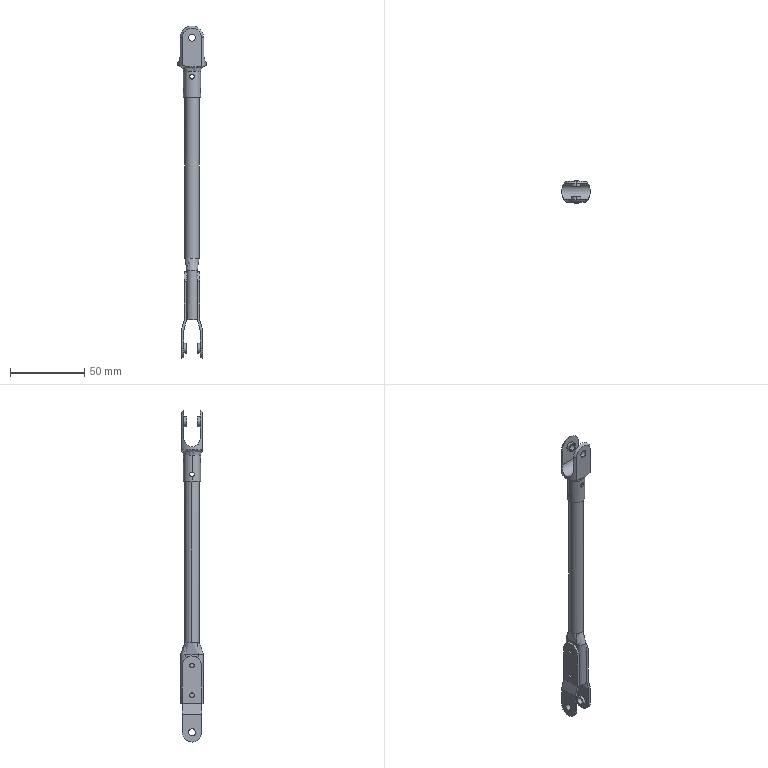Part | SolidWorks | features BaseBody 2 | 2 solids | 108 faces | box 19.177 x 15.419 x 223.764 mm | volume 9141 mm3 | cylinder 59 | plane 38 | spline 11 | commonest cylinder face diameters 3.175 x16 3.183 x8 4.826 x8 6.604 x8 13 x6 7.137 x2